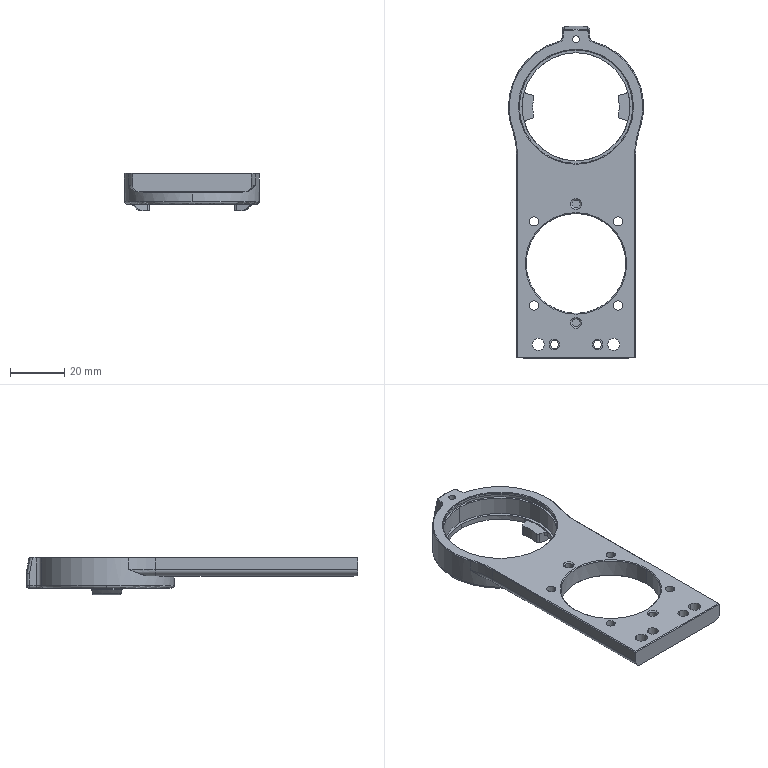NC program | NX | posted with a generic post | part box 50 x 122.9 x 14 mm
Lines 1 to 18 of 4462:
N10 G17 G21 G94 G90
(FLOOR_WALL , TOOL : D80)
N12 T19 M6
N14 G54
N16 G17 G0 G90 X-106.45 Y0. S5000 M3
N18 G43 Z30. H19
N20 Z3.
N22 G94 G1 Z0. F1200.
N24 X-103.45
N26 X103.45
N28 X106.45
N30 Z3.
N32 G0 Z30.
N34 M5